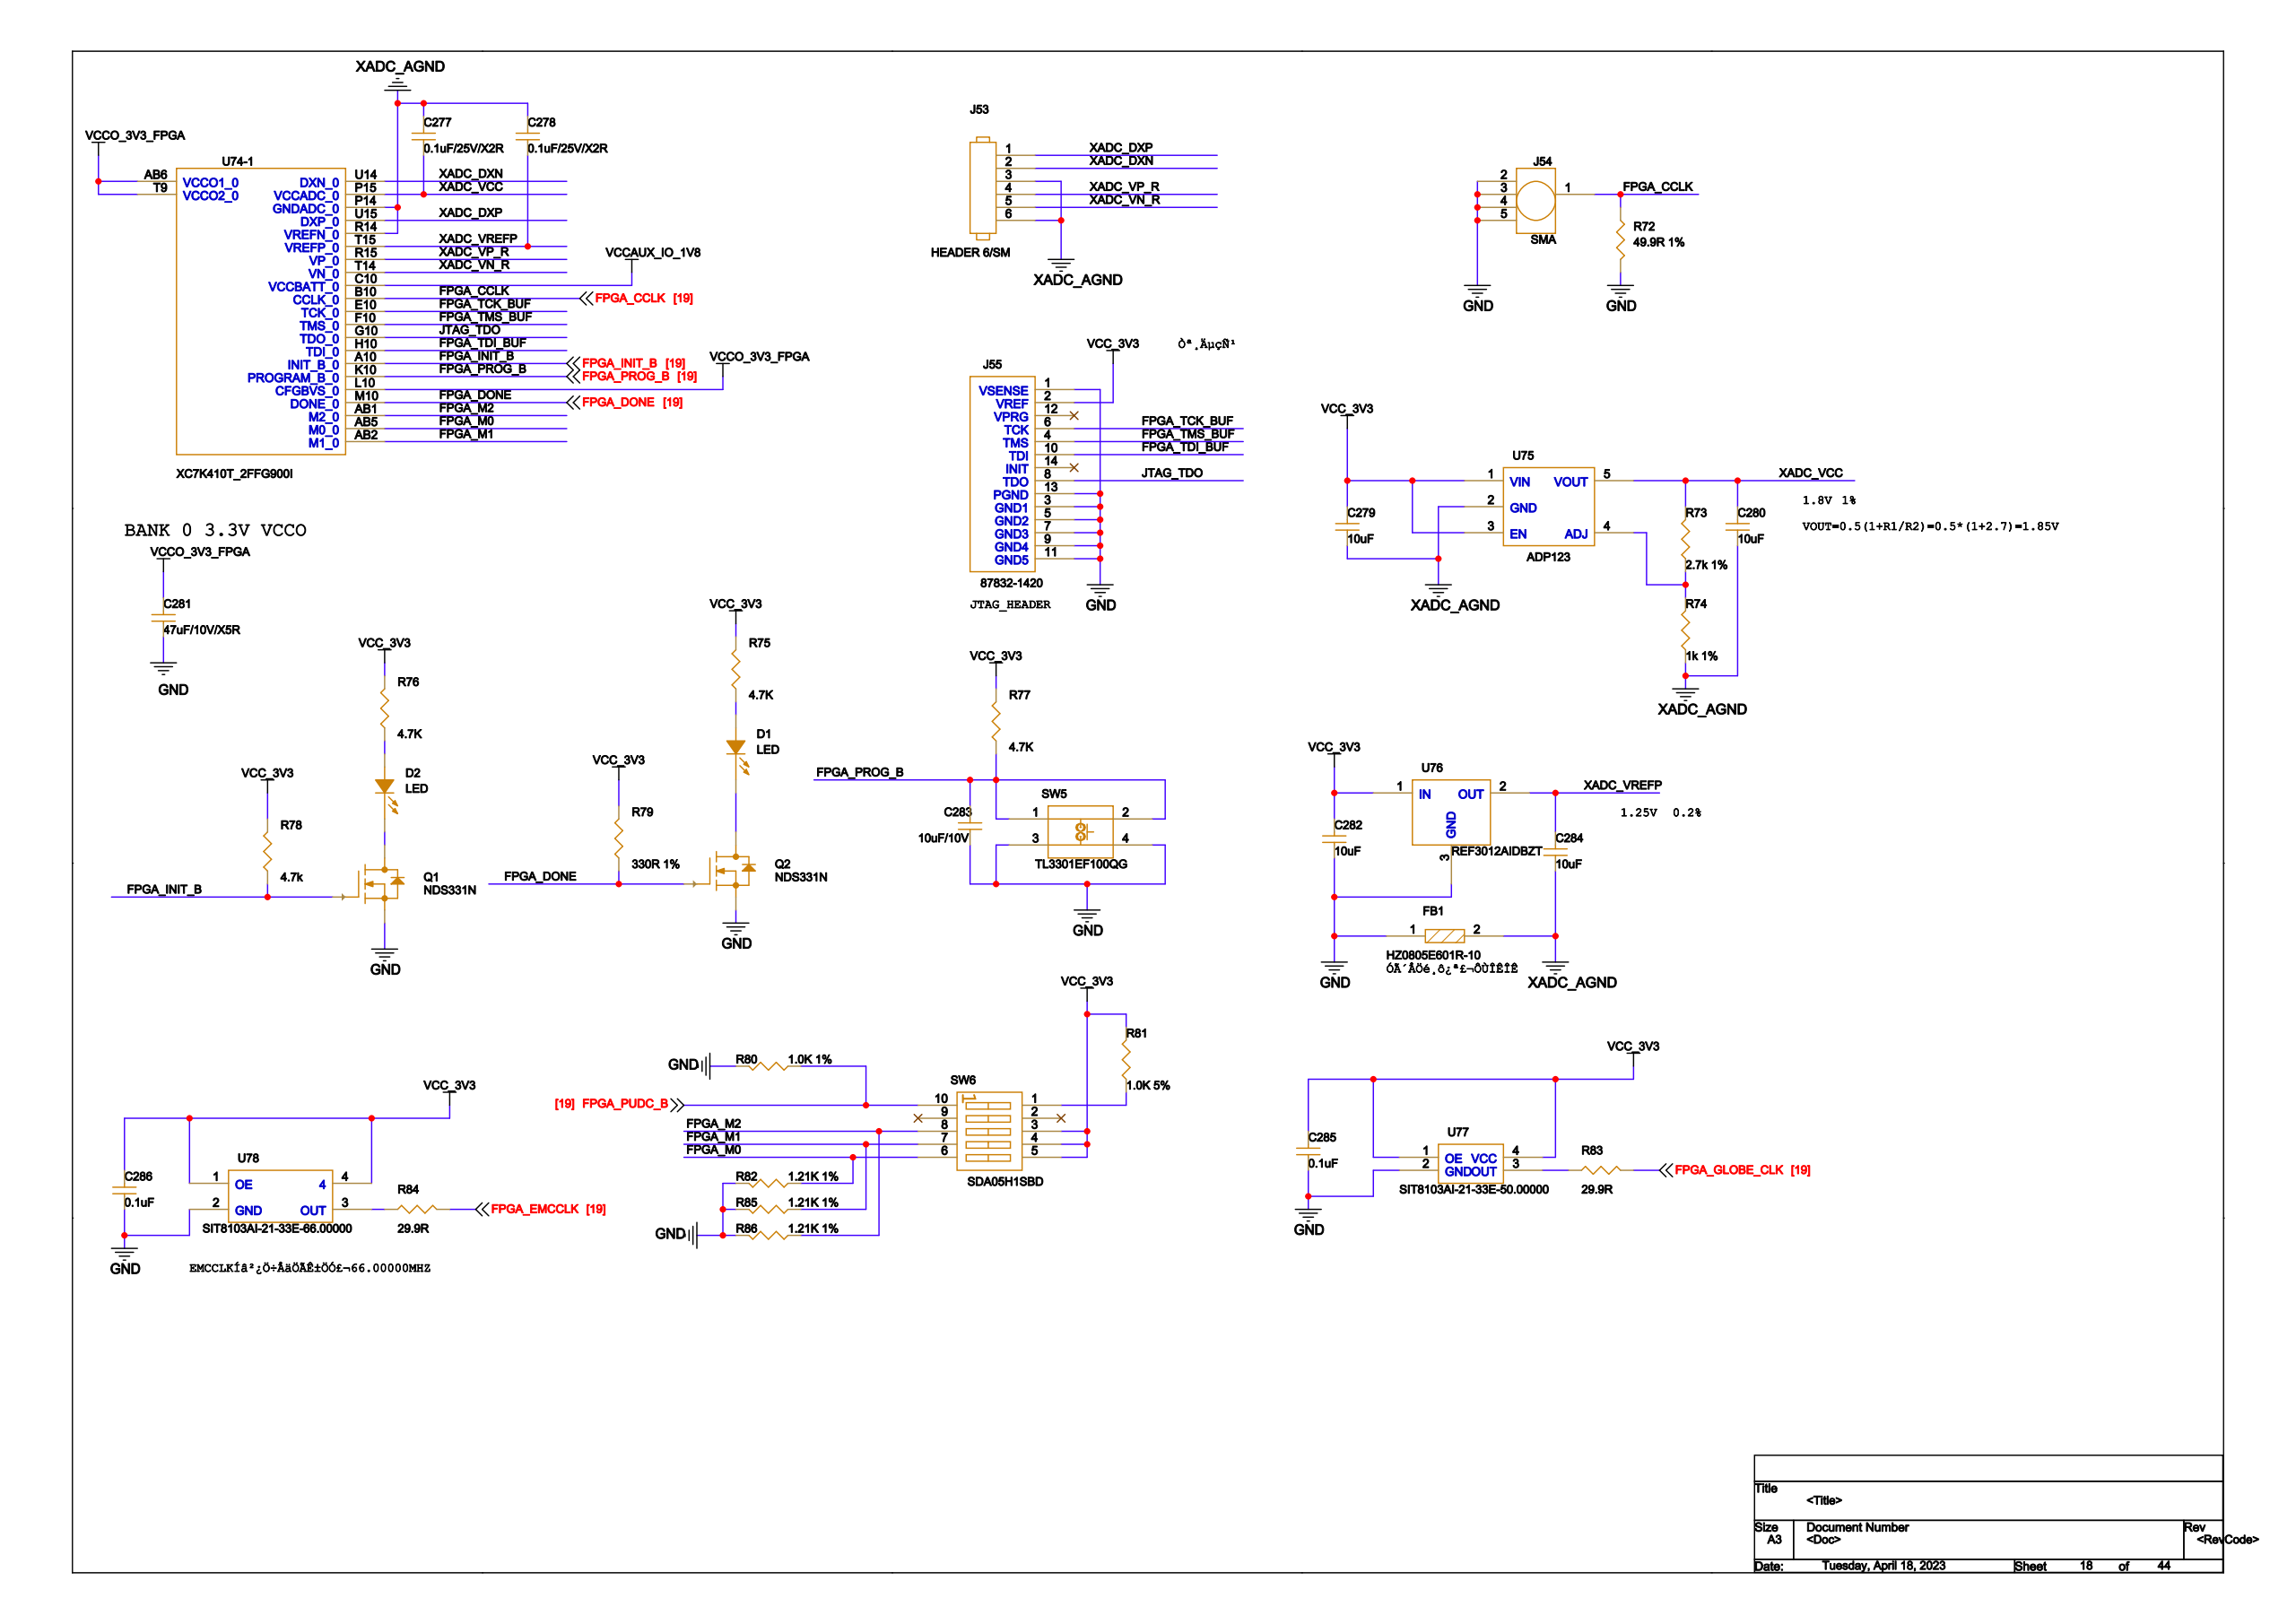Circuit board | Cadence Allegro | 1034 parts | 912 nets | one sheet of the schematic
Parts on this sheet (reference | value | footprint):
C277 | 0.1uF/25V/X2R | C0402_BGA
C278 | 0.1uF/25V/X2R | C0402_BGA
C279 | 10uF | C0402
C280 | 10uF | C0402
C281 | 47uF/10V/X5R | C0402_BGA
C282 | 10uF | C0402
C283 | 10uF/10V | C0402
C284 | 10uF | C0402
C285 | 0.1uF | C0402
C286 | 0.1uF | C0402
FB1 | HZ0805E601R-10 | HZ0805
J53 | HEADER 6/SM | HEADER6X1-2_54
J54 | SMA | 32K10K_400
J55 | 87832-1420 | HEADER2X7_2MM54
Q1 | NDS331N | MOS_SOT23
Q2 | NDS331N | MOS_SOT23
R72 | 49.9R 1% | R0402
R73 | 2.7k 1% | R0402
R74 | 1k 1% | R0402
R75 | 4.7k | R0402
R76 | 4.7k | R0402
R77 | 4.7k | R0402
R78 | 4.7k | R0402
R79 | 330R 1% | R0402
R80 | 1.0K 1% | R0402
R81 | 1.0K 5% | R0402
R82 | 1.21K 1% | R0402
R83 | 29.9R | R0402
R84 | 29.9R | R0402
R85 | 1.21K 1% | R0402
R86 | 1.21K 1% | R0402
SW5 | TL3301EF100QG | GULLWING4
SW6 | SDA05H1SBD | SDA05_SMD
U75 | ADP123 | ADP123_TSOT5
U76 | REF3012AIDBZT | REF3012_SOT23
U77 | SIT8103AI-21-33E-50 | SIT_3MM2X2MM5
U78 | SIT8103AI-21-33E-66 | SIT_3MM2X2MM5
Nets of these parts (net: part-pin ...):
GND: C281-1 C282-1 C283-1 C285-1 C286-1 FB1-1 J54-2 J54-3 J54-4 J54-5 J55-1 J55-3 J55-5 J55-7 J55-9 J55-11 J55-13 Q1-2 Q2-2 R72-1 R80-2 R82-2 R85-2 R86-2 SW5-3 SW5-4 U76-3 U77-2 U78-2
FPGA_TCK_BUF: J55-6
FPGA_TDI_BUF: J55-10
JTAG_TDO: J55-8
FPGA_TMS_BUF: J55-4
VCC_3V3: C279-2 C282-2 C285-2 C286-2 J55-2 R75-2 R76-2 R77-2 R78-2 R79-2 R81-2 SW6-3 SW6-4 SW6-5 U75-1 U75-3 U76-1 U77-1 U77-4 U78-1 U78-4
FPGA_PUDC_B: R80-1 SW6-10
XADC_DXP: J53-1
XADC_DXN: J53-2
XADC_AGND: C277-2 C278-2 C279-1 C280-1 C284-1 FB1-2 J53-3 J53-6 R74-1 U75-2
XADC_VP_R: J53-4
XADC_VN_R: J53-5
XADC_VCC: C277-1 C280-2 R73-2 U75-5
XADC_VREFP: C278-1 C284-2 U76-2
VCCO_3V3_FPGA: C281-2
N172368: R81-1 SW6-1
N13758068: R84-1 U78-3
FPGA_PROG_B: C283-2 R77-1 SW5-1 SW5-2
N13919114: R75-1
N13919108: Q2-3
N13919672: R76-1
N13919720: Q1-3
FPGA_CCLK: J54-1 R72-2
FPGA_INIT_B: Q1-1 R78-1
FPGA_DONE: Q2-1 R79-1
N14075791: R83-1 U77-3
FPGA_GLOBE_CLK: R83-2
FPGA_EMCCLK: R84-2
N13754403: R73-1 R74-2 U75-4
FPGA_M0: R82-1 SW6-6
FPGA_M1: R85-1 SW6-7
FPGA_M2: R86-1 SW6-8